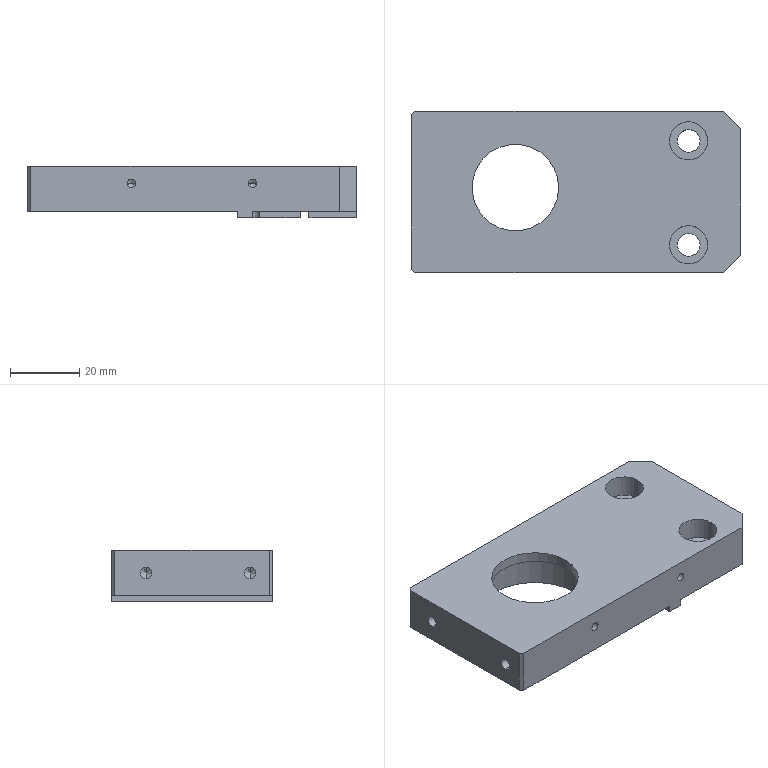Part | 1 solid | 67 faces | box 95 x 46.5 x 15 mm | volume 46606 mm3 | plane 31 | cylinder 28 | cone 8 | commonest cylinder face diameters 4 x8 2.5 x4 3.3 x4 6.6 x4 11 x4 25 x2